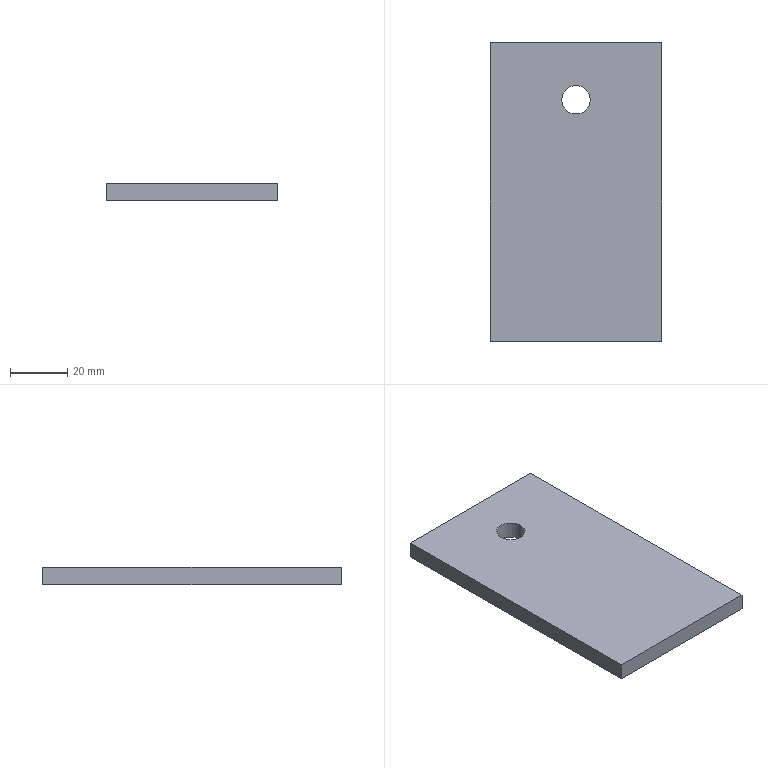Part | SolidWorks | features FlatPattern 1, SMBaseFlange 1, SheetMetal 1 | 1 solid | 8 faces | box 60 x 104.7 x 6 mm | volume 37221 mm3 | plane 6 | cylinder 2 | commonest cylinder face diameters 10 x2
STEP:
#1=CARTESIAN_POINT('',(25.,84.7,-6.));
#2=VERTEX_POINT('',#1);
#3=CARTESIAN_POINT('',(35.,84.7,-6.));
#4=VERTEX_POINT('',#3);
#5=CARTESIAN_POINT('',(30.,84.7,-6.));
#6=DIRECTION('',(0.,0.,1.));
#7=DIRECTION('',(1.,0.,0.));
#8=AXIS2_PLACEMENT_3D('',#5,#6,#7);
#9=CIRCLE('',#8,5.);
#10=EDGE_CURVE('',#2,#4,#9,.T.);
#11=ORIENTED_EDGE('',*,*,#10,.F.);
#12=CARTESIAN_POINT('',(25.,84.7,0.));
#13=VERTEX_POINT('',#12);
#14=CARTESIAN_POINT('',(25.,84.7,-6.));
#15=DIRECTION('',(0.,0.,1.));
#16=VECTOR('',#15,1000.);
#17=LINE('',#14,#16);
#18=EDGE_CURVE('',#2,#13,#17,.T.);
#19=ORIENTED_EDGE('',*,*,#18,.T.);
#20=CARTESIAN_POINT('',(35.,84.7,0.));
#21=VERTEX_POINT('',#20);
#22=CARTESIAN_POINT('',(30.,84.7,0.));
#23=DIRECTION('',(0.,0.,1.));
#24=DIRECTION('',(1.,0.,0.));
#25=AXIS2_PLACEMENT_3D('',#22,#23,#24);
#26=CIRCLE('',#25,5.);
#27=EDGE_CURVE('',#13,#21,#26,.T.);
#28=ORIENTED_EDGE('',*,*,#27,.T.);
#29=CARTESIAN_POINT('',(35.,84.7,-6.));
#30=DIRECTION('',(0.,0.,1.));
#31=VECTOR('',#30,1000.);
#32=LINE('',#29,#31);
#33=EDGE_CURVE('',#4,#21,#32,.T.);
#34=ORIENTED_EDGE('',*,*,#33,.F.);
#35=EDGE_LOOP('',(#11,#19,#28,#34));
#36=FACE_OUTER_BOUND('',#35,.T.);
#37=CARTESIAN_POINT('',(30.,84.7,-6.));
#38=DIRECTION('',(0.,0.,1.));
#39=DIRECTION('',(1.,0.,0.));
#40=AXIS2_PLACEMENT_3D('',#37,#38,#39);
#41=CYLINDRICAL_SURFACE('',#40,5.);
#42=ADVANCED_FACE('',(#36),#41,.F.);
#43=CARTESIAN_POINT('',(0.,104.7,0.));
#44=VERTEX_POINT('',#43);
#45=CARTESIAN_POINT('',(0.,0.,0.));
#46=VERTEX_POINT('',#45);
#47=CARTESIAN_POINT('',(0.,0.,0.));
#48=DIRECTION('',(0.,-1.,0.));
#49=VECTOR('',#48,1000.);
#50=LINE('',#47,#49);
#51=EDGE_CURVE('',#44,#46,#50,.T.);
#52=ORIENTED_EDGE('',*,*,#51,.F.);
#53=CARTESIAN_POINT('',(0.,104.7,-6.));
#54=VERTEX_POINT('',#53);
#55=CARTESIAN_POINT('',(0.,104.7,-6.));
#56=DIRECTION('',(0.,0.,1.));
#57=VECTOR('',#56,1000.);
#58=LINE('',#55,#57);
#59=EDGE_CURVE('',#54,#44,#58,.T.);
#60=ORIENTED_EDGE('',*,*,#59,.F.);
#61=CARTESIAN_POINT('',(0.,0.,-6.));
#62=VERTEX_POINT('',#61);
#63=CARTESIAN_POINT('',(0.,0.,-6.));
#64=DIRECTION('',(0.,-1.,0.));
#65=VECTOR('',#64,1000.);
#66=LINE('',#63,#65);
#67=EDGE_CURVE('',#54,#62,#66,.T.);
#68=ORIENTED_EDGE('',*,*,#67,.T.);
#69=CARTESIAN_POINT('',(0.,0.,-6.));
#70=DIRECTION('',(0.,0.,1.));
#71=VECTOR('',#70,1000.);
#72=LINE('',#69,#71);
#73=EDGE_CURVE('',#62,#46,#72,.T.);
#74=ORIENTED_EDGE('',*,*,#73,.T.);
#75=EDGE_LOOP('',(#52,#60,#68,#74));
#76=FACE_OUTER_BOUND('',#75,.T.);
#77=CARTESIAN_POINT('',(0.,0.,-6.));
#78=DIRECTION('',(-1.,0.,0.));
#79=DIRECTION('',(0.,0.,1.));
#80=AXIS2_PLACEMENT_3D('',#77,#78,#79);
#81=PLANE('',#80);
#82=ADVANCED_FACE('',(#76),#81,.T.);
#83=CARTESIAN_POINT('',(60.,104.7,0.));
#84=VERTEX_POINT('',#83);
#85=CARTESIAN_POINT('',(0.,104.7,0.));
#86=DIRECTION('',(-1.,0.,0.));
#87=VECTOR('',#86,1000.);
#88=LINE('',#85,#87);
#89=EDGE_CURVE('',#84,#44,#88,.T.);
#90=ORIENTED_EDGE('',*,*,#89,.F.);
#91=CARTESIAN_POINT('',(60.,104.7,-6.));
#92=VERTEX_POINT('',#91);
#93=CARTESIAN_POINT('',(60.,104.7,-6.));
#94=DIRECTION('',(0.,0.,1.));
#95=VECTOR('',#94,1000.);
#96=LINE('',#93,#95);
#97=EDGE_CURVE('',#92,#84,#96,.T.);
#98=ORIENTED_EDGE('',*,*,#97,.F.);
#99=CARTESIAN_POINT('',(0.,104.7,-6.));
#100=DIRECTION('',(-1.,0.,0.));
#101=VECTOR('',#100,1000.);
#102=LINE('',#99,#101);
#103=EDGE_CURVE('',#92,#54,#102,.T.);
#104=ORIENTED_EDGE('',*,*,#103,.T.);
#105=ORIENTED_EDGE('',*,*,#59,.T.);
#106=EDGE_LOOP('',(#90,#98,#104,#105));
#107=FACE_OUTER_BOUND('',#106,.T.);
#108=CARTESIAN_POINT('',(0.,104.7,-6.));
#109=DIRECTION('',(0.,1.,0.));
#110=DIRECTION('',(0.,0.,1.));
#111=AXIS2_PLACEMENT_3D('',#108,#109,#110);
#112=PLANE('',#111);
#113=ADVANCED_FACE('',(#107),#112,.T.);
#114=CARTESIAN_POINT('',(60.,0.,0.));
#115=VERTEX_POINT('',#114);
#116=CARTESIAN_POINT('',(60.,0.,0.));
#117=DIRECTION('',(0.,1.,0.));
#118=VECTOR('',#117,1000.);
#119=LINE('',#116,#118);
#120=EDGE_CURVE('',#115,#84,#119,.T.);
#121=ORIENTED_EDGE('',*,*,#120,.F.);
#122=CARTESIAN_POINT('',(60.,0.,-6.));
#123=VERTEX_POINT('',#122);
#124=CARTESIAN_POINT('',(60.,0.,-6.));
#125=DIRECTION('',(0.,0.,1.));
#126=VECTOR('',#125,1000.);
#127=LINE('',#124,#126);
#128=EDGE_CURVE('',#123,#115,#127,.T.);
#129=ORIENTED_EDGE('',*,*,#128,.F.);
#130=CARTESIAN_POINT('',(60.,0.,-6.));
#131=DIRECTION('',(0.,1.,0.));
#132=VECTOR('',#131,1000.);
#133=LINE('',#130,#132);
#134=EDGE_CURVE('',#123,#92,#133,.T.);
#135=ORIENTED_EDGE('',*,*,#134,.T.);
#136=ORIENTED_EDGE('',*,*,#97,.T.);
#137=EDGE_LOOP('',(#121,#129,#135,#136));
#138=FACE_OUTER_BOUND('',#137,.T.);
#139=CARTESIAN_POINT('',(60.,0.,-6.));
#140=DIRECTION('',(1.,0.,0.));
#141=DIRECTION('',(0.,0.,-1.));
#142=AXIS2_PLACEMENT_3D('',#139,#140,#141);
#143=PLANE('',#142);
#144=ADVANCED_FACE('',(#138),#143,.T.);
#145=CARTESIAN_POINT('',(0.,0.,0.));
#146=DIRECTION('',(1.,0.,0.));
#147=VECTOR('',#146,1000.);
#148=LINE('',#145,#147);
#149=EDGE_CURVE('',#46,#115,#148,.T.);
#150=ORIENTED_EDGE('',*,*,#149,.F.);
#151=ORIENTED_EDGE('',*,*,#73,.F.);
#152=CARTESIAN_POINT('',(0.,0.,-6.));
#153=DIRECTION('',(1.,0.,0.));
#154=VECTOR('',#153,1000.);
#155=LINE('',#152,#154);
#156=EDGE_CURVE('',#62,#123,#155,.T.);
#157=ORIENTED_EDGE('',*,*,#156,.T.);
#158=ORIENTED_EDGE('',*,*,#128,.T.);
#159=EDGE_LOOP('',(#150,#151,#157,#158));
#160=FACE_OUTER_BOUND('',#159,.T.);
#161=CARTESIAN_POINT('',(0.,0.,-6.));
#162=DIRECTION('',(0.,-1.,0.));
#163=DIRECTION('',(0.,0.,-1.));
#164=AXIS2_PLACEMENT_3D('',#161,#162,#163);
#165=PLANE('',#164);
#166=ADVANCED_FACE('',(#160),#165,.T.);
#167=CARTESIAN_POINT('',(30.,84.7,-6.));
#168=DIRECTION('',(0.,0.,1.));
#169=DIRECTION('',(1.,0.,0.));
#170=AXIS2_PLACEMENT_3D('',#167,#168,#169);
#171=CIRCLE('',#170,5.);
#172=EDGE_CURVE('',#4,#2,#171,.T.);
#173=ORIENTED_EDGE('',*,*,#172,.T.);
#174=ORIENTED_EDGE('',*,*,#10,.T.);
#175=EDGE_LOOP('',(#173,#174));
#176=FACE_BOUND('',#175,.T.);
#177=ORIENTED_EDGE('',*,*,#67,.F.);
#178=ORIENTED_EDGE('',*,*,#103,.F.);
#179=ORIENTED_EDGE('',*,*,#134,.F.);
#180=ORIENTED_EDGE('',*,*,#156,.F.);
#181=EDGE_LOOP('',(#177,#178,#179,#180));
#182=FACE_OUTER_BOUND('',#181,.T.);
#183=CARTESIAN_POINT('',(0.,0.,-6.));
#184=DIRECTION('',(0.,0.,-1.));
#185=DIRECTION('',(-1.,0.,0.));
#186=AXIS2_PLACEMENT_3D('',#183,#184,#185);
#187=PLANE('',#186);
#188=ADVANCED_FACE('',(#176,#182),#187,.T.);
#189=CARTESIAN_POINT('',(30.,84.7,0.));
#190=DIRECTION('',(0.,0.,1.));
#191=DIRECTION('',(1.,0.,0.));
#192=AXIS2_PLACEMENT_3D('',#189,#190,#191);
#193=CIRCLE('',#192,5.);
#194=EDGE_CURVE('',#21,#13,#193,.T.);
#195=ORIENTED_EDGE('',*,*,#194,.F.);
#196=ORIENTED_EDGE('',*,*,#27,.F.);
#197=EDGE_LOOP('',(#195,#196));
#198=FACE_BOUND('',#197,.T.);
#199=ORIENTED_EDGE('',*,*,#51,.T.);
#200=ORIENTED_EDGE('',*,*,#149,.T.);
#201=ORIENTED_EDGE('',*,*,#120,.T.);
#202=ORIENTED_EDGE('',*,*,#89,.T.);
#203=EDGE_LOOP('',(#199,#200,#201,#202));
#204=FACE_OUTER_BOUND('',#203,.T.);
#205=CARTESIAN_POINT('',(0.,0.,0.));
#206=DIRECTION('',(0.,0.,-1.));
#207=DIRECTION('',(-1.,0.,0.));
#208=AXIS2_PLACEMENT_3D('',#205,#206,#207);
#209=PLANE('',#208);
#210=ADVANCED_FACE('',(#198,#204),#209,.F.);
#211=ORIENTED_EDGE('',*,*,#18,.F.);
#212=ORIENTED_EDGE('',*,*,#172,.F.);
#213=ORIENTED_EDGE('',*,*,#33,.T.);
#214=ORIENTED_EDGE('',*,*,#194,.T.);
#215=EDGE_LOOP('',(#211,#212,#213,#214));
#216=FACE_OUTER_BOUND('',#215,.T.);
#217=CARTESIAN_POINT('',(30.,84.7,-6.));
#218=DIRECTION('',(0.,0.,1.));
#219=DIRECTION('',(1.,0.,0.));
#220=AXIS2_PLACEMENT_3D('',#217,#218,#219);
#221=CYLINDRICAL_SURFACE('',#220,5.);
#222=ADVANCED_FACE('',(#216),#221,.F.);
#223=CLOSED_SHELL('',(#42,#82,#113,#144,#166,#188,#210,#222));
#224=MANIFOLD_SOLID_BREP('',#223);
#225=CARTESIAN_POINT('',(0.,0.,0.));
#226=DIRECTION('',(0.,0.,1.));
#227=DIRECTION('',(1.,0.,0.));
#228=AXIS2_PLACEMENT_3D('',#225,#226,#227);
#229=(LENGTH_UNIT()NAMED_UNIT(*)SI_UNIT(.MILLI.,.METRE.));
#230=UNCERTAINTY_MEASURE_WITH_UNIT(LENGTH_MEASURE(0.00001),#229,'','');
#231=(NAMED_UNIT(*)PLANE_ANGLE_UNIT()SI_UNIT($,.RADIAN.));
#232=(NAMED_UNIT(*)SI_UNIT($,.STERADIAN.)SOLID_ANGLE_UNIT());
#233=(GEOMETRIC_REPRESENTATION_CONTEXT(3)GLOBAL_UNCERTAINTY_ASSIGNED_CONTEXT((#230))GLOBAL_UNIT_ASSIGNED_CONTEXT((#229,#231,#232))REPRESENTATION_CONTEXT('',''));
#234=ADVANCED_BREP_SHAPE_REPRESENTATION('',(#224,#228),#233);